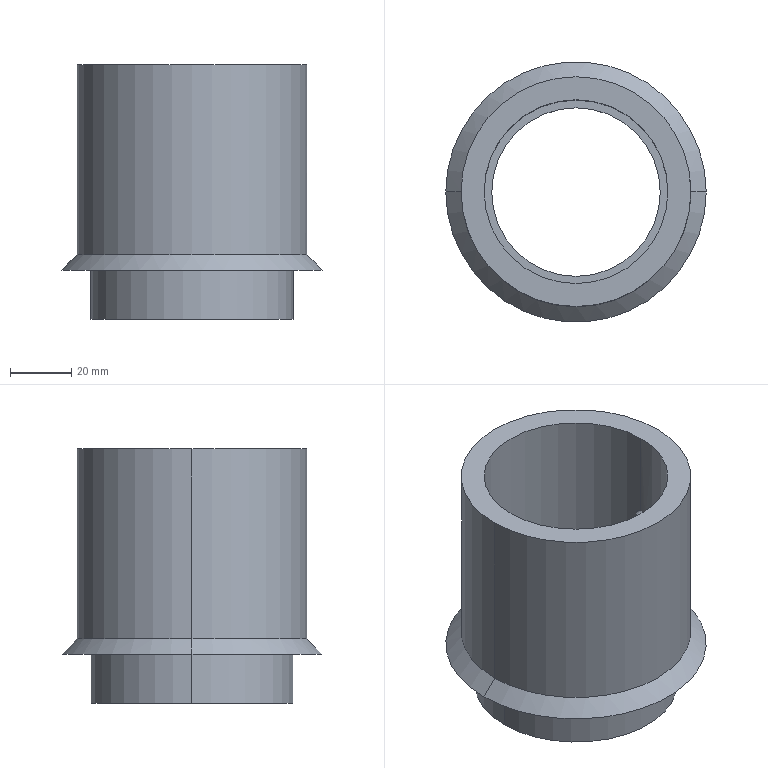Part | STEP file | Linear bearing sleeve SGN-2-11 | 1 solid | 16 faces | box 85 x 85 x 83 mm | volume 120386 mm3 | cylinder 10 | plane 4 | cone 2 | commonest cylinder face diameters 4.2 x2 55 x2 60 x2 66 x2 75 x2